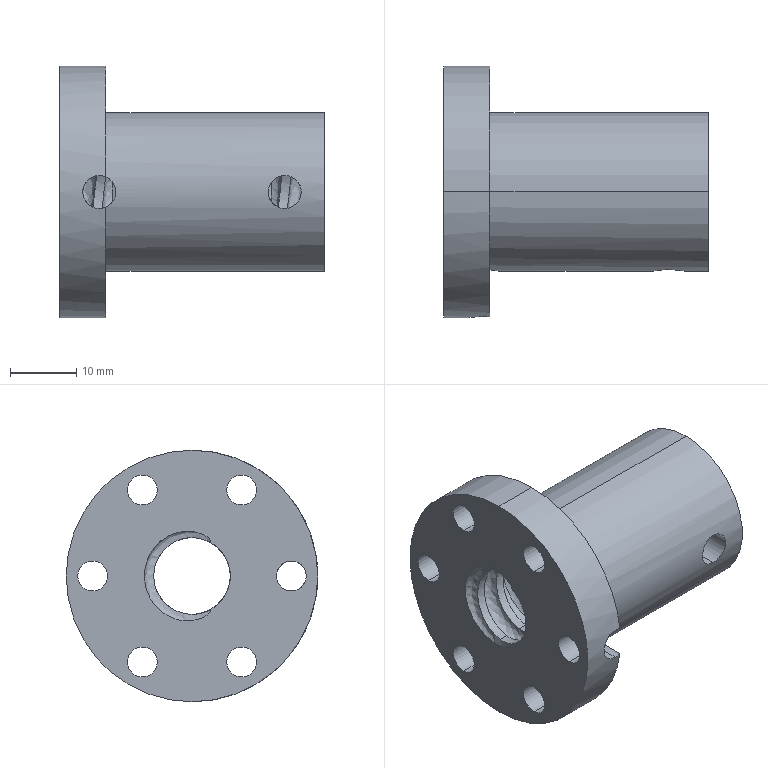Part | SolidWorks | features BaseBody 1 | 1 solid | 61 faces | box 40 x 38 x 38 mm | volume 16524 mm3 | cylinder 49 | spline 7 | plane 5 | commonest cylinder face diameters 11.6 x21 4.5 x12 5 x12 24 x2 38 x2